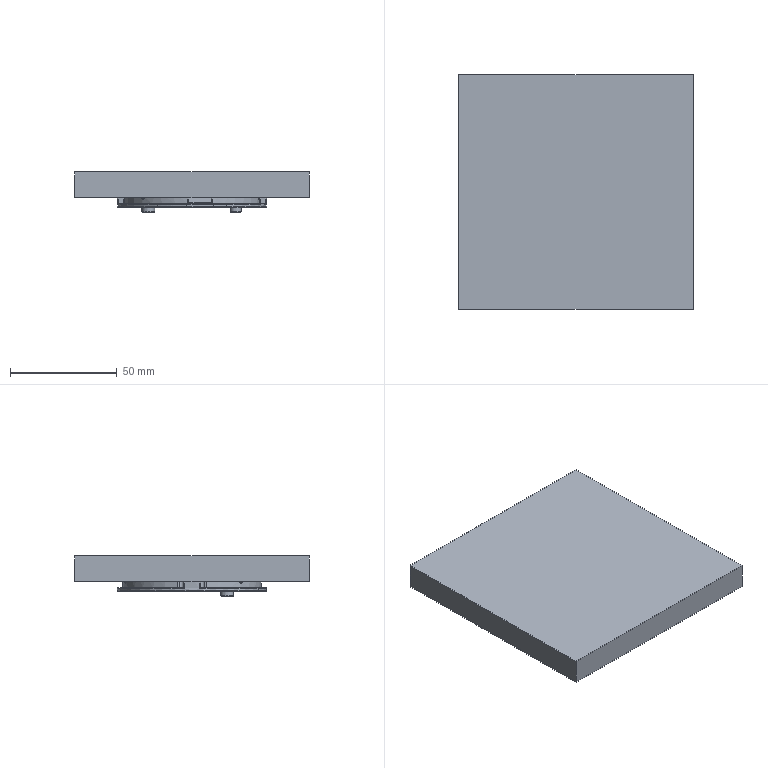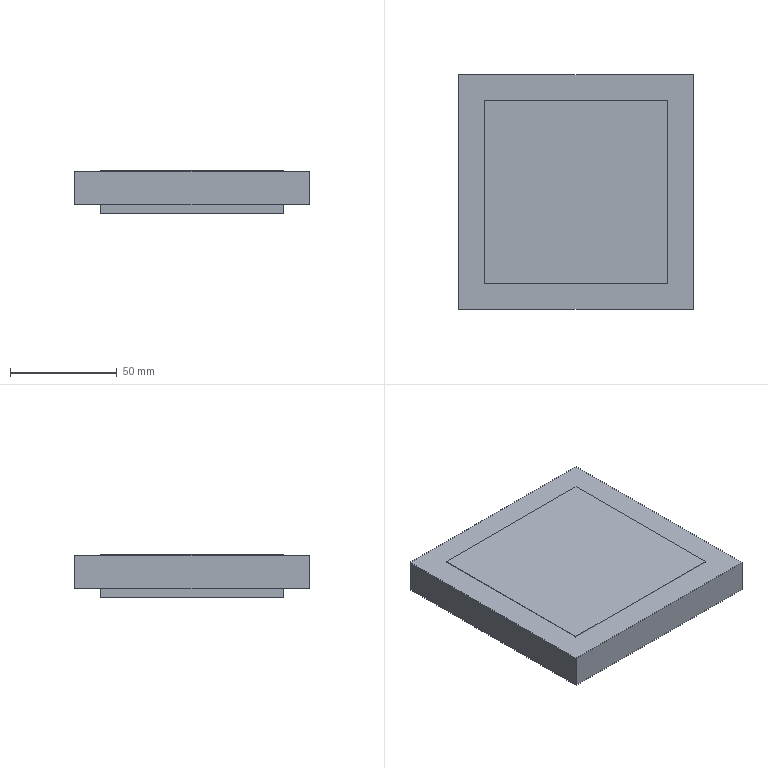CAM job | NX | 3-axis milling, drilling | part box 110 x 110 x 18.8 mm | stock box 110 x 110 x 20.3 mm
Tools:
number,name,description,diameter,corner_radius,flute_length,length,flutes
3,D63,Milling Tool-5 Parameters,63.0,0.0,50.0,75.0,2
4,D10,Milling Tool-5 Parameters,10.0,0.0,50.0,75.0,2
16,D6,Milling Tool-5 Parameters,6.0,0.0,50.0,75.0,2
17,D3,Milling Tool-5 Parameters,3.0,0.0,50.0,75.0,2
2,D2,Milling Tool-5 Parameters,2.0,0.0,50.0,75.0,2
21,D4A45,Milling Tool-5 Parameters,4.0,0.0,2.0,2.0,2
12,2.5ZT,Drilling Tool,2.5,0.0,35.0,50.0,2
13,R0.75,Milling Tool-5 Parameters,0.5,0.25,50.0,75.0,2
Operations:
program,operation,operation_type,tool,method,geometry_group,spindle_rpm,surface_speed,feed_per_tooth,feed_cut,feed_plunge,cut_length_mm,path_length_mm,cut_time_min,machine_time_min
1,FLOOR_WALL,VolumeBased25DMillingOperation,D63,METHOD,A,6500.0,1286.0,0.0962,1250.0,100.0,519.797,573.797,0.4158,0.4212
1,CAVITY_MILL,CavityMilling,D10,METHOD,A,9500.0,298.0,0.1579,3000.0,1000.0,24183.229,25793.115,8.283,8.444
1,CAVITY_MILL_COPY_1,CavityMilling,D6,METHOD,A,9500.0,179.0,0.0842,1600.0,1000.0,2081.285,3606.581,1.62,1.772
1,ZLEVEL_PROFILE,ZLevelMilling,D6,METHOD,A,9500.0,179.0,0.0526,1000.0,100.0,244.065,333.665,0.2441,0.253
1,CAVITY_MILL_COPY_1_COPY,CavityMilling,D3,METHOD,A,9500.0,89.0,0.0579,1100.0,1000.0,3613.982,5792.826,3.352,3.57
1,ZLEVEL_PROFILE_COPY_1,ZLevelMilling,D3,METHOD,A,9500.0,179.0,0.0526,1000.0,100.0,115.329,183.329,0.1153,0.1221
1,FLOOR_WALL_1,VolumeBased25DMillingOperation,D3,METHOD,A,9500.0,89.0,0.0526,1000.0,100.0,3561.72,5980.363,3.562,3.804
1,CAVITY_MILL_COPY_1_COPY_COPY,CavityMilling,D2,METHOD,A,9500.0,59.0,0.0526,1000.0,1000.0,1154.319,2428.884,1.154,1.282
1,ZLEVEL_PROFILE_COPY,ZLevelMilling,D4A45,METHOD,A,9500.0,179.0,0.0526,1000.0,100.0,111.439,171.439,0.1114,0.1174
1,ZLEVEL_PROFILE_COPY_COPY,ZLevelMilling,D4A45,METHOD,A,9500.0,179.0,0.0526,1000.0,100.0,329.659,753.567,0.3297,0.372
1,ZLEVEL_PROFILE_COPY_COPY_COPY_1,ZLevelMilling,D4A45,METHOD,A,9500.0,179.0,0.0526,1000.0,100.0,29.716,179.913,0.0297,0.0447
1,ZLEVEL_PROFILE_COPY_COPY_COPY,ZLevelMilling,D4A45,METHOD,A,9500.0,179.0,0.0526,1000.0,100.0,73.445,473.39,0.0734,0.1134
1,ZLEVEL_PROFILE_COPY_COPY_COPY_COPY_COPY,ZLevelMilling,D4A45,METHOD,MCS_MILL-A,9500.0,179.0,0.0526,1000.0,100.0,272.52,895.742,0.2725,0.3348
1,CUTTERCOMP2,ZLevelMilling,D2,METHOD,A,9500.0,179.0,0.0526,1000.0,100.0,91.07,849.65,0.0911,0.1669
1,DRILLING_1,HoleDrilling,D4A45,METHOD,A,5000.0,62.0,0.025,250.0,0.0,25.505,373.447,0.051,0.0858
1,DRILLING_1_COPY,HoleDrilling,2.5ZT,METHOD,A,2000.0,15.0,0.03,120.0,0.0,181.066,529.013,0.2294,0.2642
2,ZLEVEL_PROFILE_1,ZLevelMilling,D10,METHOD,MCS_MILL_B,9500.0,298.0,0.1053,2000.0,1000.0,1376.638,1430.038,0.7118,0.7172
2,FLOOR_WALL_COPY,VolumeBased25DMillingOperation,D63,METHOD,B,6500.0,1286.0,0.0962,1250.0,100.0,2598.525,3516.38,2.079,2.171
2,DRILLING,Operation,D4A45,METHOD,B,5000.0,94.0,0.025,250.0,0.0,8.0,120.11,0.032,0.0432
2,DRILLING_COPY,Operation,2.5ZT,METHOD,B,2000.0,15.0,0.0375,150.0,0.0,20.802,145.714,0.1387,0.1512
2,FLOOR_WALL_2,VolumeBased25DMillingOperation,D10,METHOD,B,9500.0,298.0,0.1316,2500.0,1000.0,2913.447,3034.718,1.182,1.194
2,ZLEVEL_PROFILE_1_COPY,ZLevelMilling,D10,METHOD,B,9500.0,298.0,0.0789,1500.0,1000.0,216.894,285.494,0.1464,0.1532
2,FLOOR_WALL_1_COPY,VolumeBased25DMillingOperation,D3,METHOD,B,9500.0,89.0,0.0526,1000.0,100.0,2959.431,3232.517,2.959,2.987
2,ZLEVEL_PROFILE_1_COPY_1_COPY,ZLevelMilling,D3,METHOD,B,9500.0,59.0,0.0526,1000.0,1000.0,724.736,800.336,0.7247,0.7323
2,ZLEVEL_PROFILE_1_COPY_1_COPY_COPY,ZLevelMilling,D2,METHOD,B,9500.0,59.0,0.0526,1000.0,1000.0,1096.797,1172.397,1.097,1.104
2,ZLEVEL_PROFILE_1_COPY_1,ZLevelMilling,D2,METHOD,B,9500.0,59.0,0.0526,1000.0,1000.0,12008.047,12237.974,12.008,12.031
2,ZLEVEL_PROFILE_COPY_COPY_COPY_1_COPY,ZLevelMilling,D4A45,METHOD,B,9500.0,179.0,0.0526,1000.0,100.0,62.382,395.81,0.0624,0.0957
2,ZLEVEL_PROFILE_COPY_COPY_COPY_1_COPY_COPY,ZLevelMilling,D4A45,METHOD,B,9500.0,179.0,0.0526,1000.0,100.0,481.731,830.913,0.4817,0.5166
2,ZLEVEL_PROFILE_COPY_COPY_COPY_1_COPY_COPY_COPY,ZLevelMilling,D4A45,METHOD,B,9500.0,179.0,0.0526,1000.0,100.0,32.718,174.725,0.0327,0.0469
2,ZLEVEL_PROFILE_1_COPY_1_COPY_1,ZLevelMilling,R0.75,METHOD,B,37561.0,59.0,0.0133,1000.0,800.0,64.023,127.923,0.0669,0.0733
2,CUTTERCOMP,VolumeBased25DMillingOperation,D3,METHOD,B,9500.0,89.0,0.0526,1000.0,100.0,67.534,243.351,0.0675,0.0851
FIXTURE3,FLOOR_WALL_COPY_1,VolumeBased25DMillingOperation,D10,METHOD,C,6500.0,1286.0,0.0962,1250.0,100.0,1917.997,1971.997,1.534,1.54
FIXTURE3,FLOOR_WALL_COPY_1_COPY,VolumeBased25DMillingOperation,D10,METHOD,C,9500.0,298.0,0.1316,2500.0,1000.0,3826.316,3919.037,1.604,1.613
FIXTURE3,CAVITY_MILL_COPY,CavityMilling,D10,METHOD,C,9500.0,298.0,0.1579,3000.0,1000.0,1509.128,1732.501,0.7884,0.8107
FIXTURE3,CAVITY_MILL_COPY_1_COPY_1,CavityMilling,D6,METHOD,C,9500.0,179.0,0.0842,1600.0,1000.0,775.999,1562.884,0.5451,0.6238
FIXTURE3,FLOOR_WALL_1_COPY_COPY,VolumeBased25DMillingOperation,D6,METHOD,C,9500.0,89.0,0.0526,1000.0,100.0,4499.005,4631.499,4.499,4.512
FIXTURE3,CAVITY_MILL_COPY_1_COPY_COPY_COPY,CavityMilling,D2,METHOD,C,9500.0,59.0,0.0526,1000.0,1000.0,10959.157,12202.708,10.959,11.084
FIXTURE3,FLOOR_WALL_1_COPY_COPY_1,VolumeBased25DMillingOperation,D2,METHOD,C,9500.0,89.0,0.0526,1000.0,100.0,1472.881,1742.769,1.473,1.5
FIXTURE3,ZLEVEL_PROFILE_COPY_COPY_1,ZLevelMilling,D4A45,METHOD,C,9500.0,179.0,0.0526,1000.0,100.0,161.22,221.22,0.1612,0.1672
FIXTURE3,CUTTERCOMP_COPY,VolumeBased25DMillingOperation,D2,METHOD,C,9500.0,89.0,0.0526,1000.0,100.0,470.943,731.159,0.4709,0.497